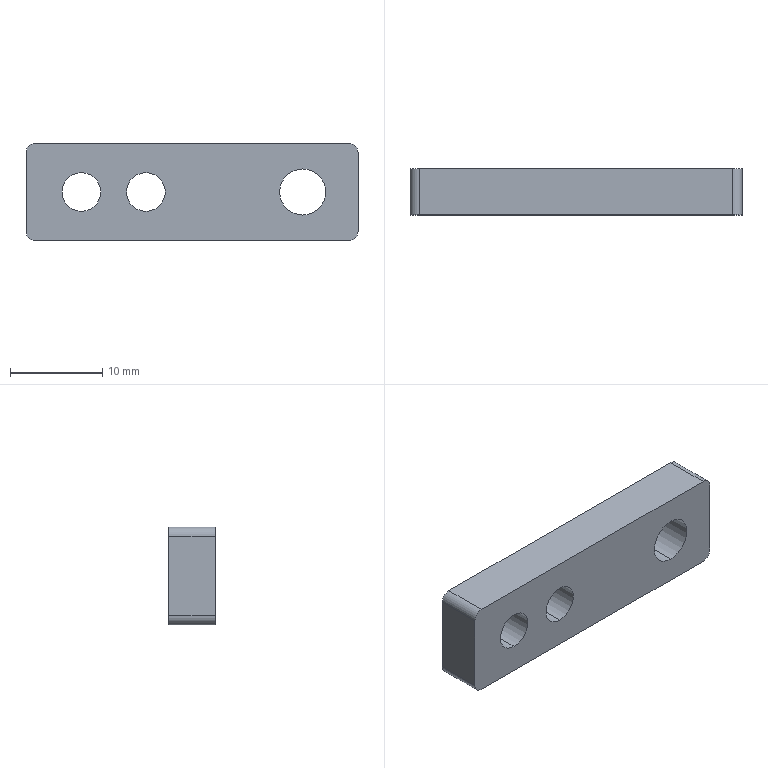Part | STEP file | Driven guide wheel connector | 1 solid | 16 faces | box 36 x 5 x 10.6 mm | volume 1667 mm3 | cylinder 10 | plane 6 | commonest cylinder face diameters 2 x4 4.2 x4 5 x2
STEP:
#1=CARTESIAN_POINT('',(0.,0.,0.));
#2=DIRECTION('',(0.,0.,1.));
#3=DIRECTION('',(1.,0.,0.));
#4=AXIS2_PLACEMENT_3D('',#1,#2,#3);
#5=CARTESIAN_POINT('',(12.,-5.,2.5));
#6=VERTEX_POINT('',#5);
#7=CARTESIAN_POINT('',(12.,0.,2.5));
#8=VERTEX_POINT('',#7);
#9=CARTESIAN_POINT('',(12.,0.,2.5));
#10=DIRECTION('',(0.,1.,0.));
#11=VECTOR('',#10,1.);
#12=LINE('',#9,#11);
#13=CARTESIAN_POINT('',(12.,0.,0.));
#14=DIRECTION('',(0.,1.,0.));
#15=DIRECTION('',(0.,0.,1.));
#16=AXIS2_PLACEMENT_3D('',#13,#14,#15);
#17=CYLINDRICAL_SURFACE('',#16,2.5);
#18=CARTESIAN_POINT('',(6.283,0.));
#19=DIRECTION('',(0.,1.));
#20=VECTOR('',#19,1.);
#21=LINE('',#18,#20);
#22=(GEOMETRIC_REPRESENTATION_CONTEXT(2)PARAMETRIC_REPRESENTATION_CONTEXT()REPRESENTATION_CONTEXT('',''));
#23=DEFINITIONAL_REPRESENTATION('',(#21),#22);
#24=PCURVE('',#17,#23);
#25=CARTESIAN_POINT('',(12.,0.,0.));
#26=DIRECTION('',(0.,1.,0.));
#27=DIRECTION('',(0.,0.,1.));
#28=AXIS2_PLACEMENT_3D('',#25,#26,#27);
#29=CYLINDRICAL_SURFACE('',#28,2.5);
#30=CARTESIAN_POINT('',(0.,0.));
#31=DIRECTION('',(0.,1.));
#32=VECTOR('',#31,1.);
#33=LINE('',#30,#32);
#34=(GEOMETRIC_REPRESENTATION_CONTEXT(2)PARAMETRIC_REPRESENTATION_CONTEXT()REPRESENTATION_CONTEXT('',''));
#35=DEFINITIONAL_REPRESENTATION('',(#33),#34);
#36=PCURVE('',#29,#35);
#37=SURFACE_CURVE('',#12,(#24,#36),.PCURVE_S1.);
#38=EDGE_CURVE('',#6,#8,#37,.T.);
#39=ORIENTED_EDGE('',*,*,#38,.T.);
#40=CARTESIAN_POINT('',(12.,0.,-2.5));
#41=VERTEX_POINT('',#40);
#42=CARTESIAN_POINT('',(12.,0.,0.));
#43=DIRECTION('',(0.,1.,0.));
#44=DIRECTION('',(0.,0.,1.));
#45=AXIS2_PLACEMENT_3D('',#42,#43,#44);
#46=CIRCLE('',#45,2.5);
#47=CARTESIAN_POINT('',(0.,0.));
#48=DIRECTION('',(1.,0.));
#49=VECTOR('',#48,1.);
#50=LINE('',#47,#49);
#51=(GEOMETRIC_REPRESENTATION_CONTEXT(2)PARAMETRIC_REPRESENTATION_CONTEXT()REPRESENTATION_CONTEXT('',''));
#52=DEFINITIONAL_REPRESENTATION('',(#50),#51);
#53=PCURVE('',#17,#52);
#54=CARTESIAN_POINT('',(0.,0.,0.));
#55=DIRECTION('',(0.,1.,0.));
#56=DIRECTION('',(0.,0.,1.));
#57=AXIS2_PLACEMENT_3D('',#54,#55,#56);
#58=PLANE('',#57);
#59=CARTESIAN_POINT('',(0.,12.));
#60=DIRECTION('',(1.,0.));
#61=AXIS2_PLACEMENT_2D('',#59,#60);
#62=CIRCLE('',#61,2.5);
#63=(GEOMETRIC_REPRESENTATION_CONTEXT(2)PARAMETRIC_REPRESENTATION_CONTEXT()REPRESENTATION_CONTEXT('',''));
#64=DEFINITIONAL_REPRESENTATION('',(#62),#63);
#65=PCURVE('',#58,#64);
#66=SURFACE_CURVE('',#46,(#53,#65),.PCURVE_S1.);
#67=EDGE_CURVE('',#41,#8,#66,.T.);
#68=ORIENTED_EDGE('',*,*,#67,.F.);
#69=CARTESIAN_POINT('',(12.,-5.,-2.5));
#70=VERTEX_POINT('',#69);
#71=CARTESIAN_POINT('',(12.,0.,-2.5));
#72=DIRECTION('',(0.,1.,0.));
#73=VECTOR('',#72,1.);
#74=LINE('',#71,#73);
#75=CARTESIAN_POINT('',(3.142,0.));
#76=DIRECTION('',(0.,1.));
#77=VECTOR('',#76,1.);
#78=LINE('',#75,#77);
#79=(GEOMETRIC_REPRESENTATION_CONTEXT(2)PARAMETRIC_REPRESENTATION_CONTEXT()REPRESENTATION_CONTEXT('',''));
#80=DEFINITIONAL_REPRESENTATION('',(#78),#79);
#81=PCURVE('',#17,#80);
#82=CARTESIAN_POINT('',(3.142,0.));
#83=DIRECTION('',(0.,1.));
#84=VECTOR('',#83,1.);
#85=LINE('',#82,#84);
#86=(GEOMETRIC_REPRESENTATION_CONTEXT(2)PARAMETRIC_REPRESENTATION_CONTEXT()REPRESENTATION_CONTEXT('',''));
#87=DEFINITIONAL_REPRESENTATION('',(#85),#86);
#88=PCURVE('',#29,#87);
#89=SURFACE_CURVE('',#74,(#81,#88),.PCURVE_S1.);
#90=EDGE_CURVE('',#70,#41,#89,.T.);
#91=ORIENTED_EDGE('',*,*,#90,.F.);
#92=CARTESIAN_POINT('',(12.,-5.,0.));
#93=DIRECTION('',(0.,1.,0.));
#94=DIRECTION('',(0.,0.,1.));
#95=AXIS2_PLACEMENT_3D('',#92,#93,#94);
#96=CIRCLE('',#95,2.5);
#97=CARTESIAN_POINT('',(0.,-5.));
#98=DIRECTION('',(1.,0.));
#99=VECTOR('',#98,1.);
#100=LINE('',#97,#99);
#101=(GEOMETRIC_REPRESENTATION_CONTEXT(2)PARAMETRIC_REPRESENTATION_CONTEXT()REPRESENTATION_CONTEXT('',''));
#102=DEFINITIONAL_REPRESENTATION('',(#100),#101);
#103=PCURVE('',#17,#102);
#104=CARTESIAN_POINT('',(0.,-5.,0.));
#105=DIRECTION('',(0.,1.,0.));
#106=DIRECTION('',(0.,0.,1.));
#107=AXIS2_PLACEMENT_3D('',#104,#105,#106);
#108=PLANE('',#107);
#109=CARTESIAN_POINT('',(0.,12.));
#110=DIRECTION('',(1.,0.));
#111=AXIS2_PLACEMENT_2D('',#109,#110);
#112=CIRCLE('',#111,2.5);
#113=(GEOMETRIC_REPRESENTATION_CONTEXT(2)PARAMETRIC_REPRESENTATION_CONTEXT()REPRESENTATION_CONTEXT('',''));
#114=DEFINITIONAL_REPRESENTATION('',(#112),#113);
#115=PCURVE('',#108,#114);
#116=SURFACE_CURVE('',#96,(#103,#115),.PCURVE_S1.);
#117=EDGE_CURVE('',#70,#6,#116,.T.);
#118=ORIENTED_EDGE('',*,*,#117,.T.);
#119=EDGE_LOOP('',(#39,#68,#91,#118));
#120=FACE_BOUND('',#119,.F.);
#121=ADVANCED_FACE('',(#120),#17,.F.);
#122=CARTESIAN_POINT('',(-5.,-5.,2.1));
#123=VERTEX_POINT('',#122);
#124=CARTESIAN_POINT('',(-5.,0.,2.1));
#125=VERTEX_POINT('',#124);
#126=CARTESIAN_POINT('',(-5.,0.,2.1));
#127=DIRECTION('',(0.,1.,0.));
#128=VECTOR('',#127,1.);
#129=LINE('',#126,#128);
#130=CARTESIAN_POINT('',(-5.,0.,0.));
#131=DIRECTION('',(0.,1.,0.));
#132=DIRECTION('',(0.,0.,1.));
#133=AXIS2_PLACEMENT_3D('',#130,#131,#132);
#134=CYLINDRICAL_SURFACE('',#133,2.1);
#135=CARTESIAN_POINT('',(6.283,0.));
#136=DIRECTION('',(0.,1.));
#137=VECTOR('',#136,1.);
#138=LINE('',#135,#137);
#139=(GEOMETRIC_REPRESENTATION_CONTEXT(2)PARAMETRIC_REPRESENTATION_CONTEXT()REPRESENTATION_CONTEXT('',''));
#140=DEFINITIONAL_REPRESENTATION('',(#138),#139);
#141=PCURVE('',#134,#140);
#142=CARTESIAN_POINT('',(-5.,0.,0.));
#143=DIRECTION('',(0.,1.,0.));
#144=DIRECTION('',(0.,0.,1.));
#145=AXIS2_PLACEMENT_3D('',#142,#143,#144);
#146=CYLINDRICAL_SURFACE('',#145,2.1);
#147=CARTESIAN_POINT('',(0.,0.));
#148=DIRECTION('',(0.,1.));
#149=VECTOR('',#148,1.);
#150=LINE('',#147,#149);
#151=(GEOMETRIC_REPRESENTATION_CONTEXT(2)PARAMETRIC_REPRESENTATION_CONTEXT()REPRESENTATION_CONTEXT('',''));
#152=DEFINITIONAL_REPRESENTATION('',(#150),#151);
#153=PCURVE('',#146,#152);
#154=SURFACE_CURVE('',#129,(#141,#153),.PCURVE_S1.);
#155=EDGE_CURVE('',#123,#125,#154,.T.);
#156=ORIENTED_EDGE('',*,*,#155,.T.);
#157=CARTESIAN_POINT('',(-5.,0.,-2.1));
#158=VERTEX_POINT('',#157);
#159=CARTESIAN_POINT('',(-5.,0.,0.));
#160=DIRECTION('',(0.,1.,0.));
#161=DIRECTION('',(0.,0.,1.));
#162=AXIS2_PLACEMENT_3D('',#159,#160,#161);
#163=CIRCLE('',#162,2.1);
#164=CARTESIAN_POINT('',(0.,0.));
#165=DIRECTION('',(1.,0.));
#166=VECTOR('',#165,1.);
#167=LINE('',#164,#166);
#168=(GEOMETRIC_REPRESENTATION_CONTEXT(2)PARAMETRIC_REPRESENTATION_CONTEXT()REPRESENTATION_CONTEXT('',''));
#169=DEFINITIONAL_REPRESENTATION('',(#167),#168);
#170=PCURVE('',#134,#169);
#171=CARTESIAN_POINT('',(0.,-5.));
#172=DIRECTION('',(1.,0.));
#173=AXIS2_PLACEMENT_2D('',#171,#172);
#174=CIRCLE('',#173,2.1);
#175=(GEOMETRIC_REPRESENTATION_CONTEXT(2)PARAMETRIC_REPRESENTATION_CONTEXT()REPRESENTATION_CONTEXT('',''));
#176=DEFINITIONAL_REPRESENTATION('',(#174),#175);
#177=PCURVE('',#58,#176);
#178=SURFACE_CURVE('',#163,(#170,#177),.PCURVE_S1.);
#179=EDGE_CURVE('',#158,#125,#178,.T.);
#180=ORIENTED_EDGE('',*,*,#179,.F.);
#181=CARTESIAN_POINT('',(-5.,-5.,-2.1));
#182=VERTEX_POINT('',#181);
#183=CARTESIAN_POINT('',(-5.,0.,-2.1));
#184=DIRECTION('',(0.,1.,0.));
#185=VECTOR('',#184,1.);
#186=LINE('',#183,#185);
#187=CARTESIAN_POINT('',(3.142,0.));
#188=DIRECTION('',(0.,1.));
#189=VECTOR('',#188,1.);
#190=LINE('',#187,#189);
#191=(GEOMETRIC_REPRESENTATION_CONTEXT(2)PARAMETRIC_REPRESENTATION_CONTEXT()REPRESENTATION_CONTEXT('',''));
#192=DEFINITIONAL_REPRESENTATION('',(#190),#191);
#193=PCURVE('',#134,#192);
#194=CARTESIAN_POINT('',(3.142,0.));
#195=DIRECTION('',(0.,1.));
#196=VECTOR('',#195,1.);
#197=LINE('',#194,#196);
#198=(GEOMETRIC_REPRESENTATION_CONTEXT(2)PARAMETRIC_REPRESENTATION_CONTEXT()REPRESENTATION_CONTEXT('',''));
#199=DEFINITIONAL_REPRESENTATION('',(#197),#198);
#200=PCURVE('',#146,#199);
#201=SURFACE_CURVE('',#186,(#193,#200),.PCURVE_S1.);
#202=EDGE_CURVE('',#182,#158,#201,.T.);
#203=ORIENTED_EDGE('',*,*,#202,.F.);
#204=CARTESIAN_POINT('',(-5.,-5.,0.));
#205=DIRECTION('',(0.,1.,0.));
#206=DIRECTION('',(0.,0.,1.));
#207=AXIS2_PLACEMENT_3D('',#204,#205,#206);
#208=CIRCLE('',#207,2.1);
#209=CARTESIAN_POINT('',(0.,-5.));
#210=DIRECTION('',(1.,0.));
#211=VECTOR('',#210,1.);
#212=LINE('',#209,#211);
#213=(GEOMETRIC_REPRESENTATION_CONTEXT(2)PARAMETRIC_REPRESENTATION_CONTEXT()REPRESENTATION_CONTEXT('',''));
#214=DEFINITIONAL_REPRESENTATION('',(#212),#213);
#215=PCURVE('',#134,#214);
#216=CARTESIAN_POINT('',(0.,-5.));
#217=DIRECTION('',(1.,0.));
#218=AXIS2_PLACEMENT_2D('',#216,#217);
#219=CIRCLE('',#218,2.1);
#220=(GEOMETRIC_REPRESENTATION_CONTEXT(2)PARAMETRIC_REPRESENTATION_CONTEXT()REPRESENTATION_CONTEXT('',''));
#221=DEFINITIONAL_REPRESENTATION('',(#219),#220);
#222=PCURVE('',#108,#221);
#223=SURFACE_CURVE('',#208,(#215,#222),.PCURVE_S1.);
#224=EDGE_CURVE('',#182,#123,#223,.T.);
#225=ORIENTED_EDGE('',*,*,#224,.T.);
#226=EDGE_LOOP('',(#156,#180,#203,#225));
#227=FACE_BOUND('',#226,.F.);
#228=ADVANCED_FACE('',(#227),#134,.F.);
#229=CARTESIAN_POINT('',(-12.,-5.,2.1));
#230=VERTEX_POINT('',#229);
#231=CARTESIAN_POINT('',(-12.,0.,2.1));
#232=VERTEX_POINT('',#231);
#233=CARTESIAN_POINT('',(-12.,0.,2.1));
#234=DIRECTION('',(0.,1.,0.));
#235=VECTOR('',#234,1.);
#236=LINE('',#233,#235);
#237=CARTESIAN_POINT('',(-12.,0.,0.));
#238=DIRECTION('',(0.,1.,0.));
#239=DIRECTION('',(0.,0.,1.));
#240=AXIS2_PLACEMENT_3D('',#237,#238,#239);
#241=CYLINDRICAL_SURFACE('',#240,2.1);
#242=CARTESIAN_POINT('',(6.283,0.));
#243=DIRECTION('',(0.,1.));
#244=VECTOR('',#243,1.);
#245=LINE('',#242,#244);
#246=(GEOMETRIC_REPRESENTATION_CONTEXT(2)PARAMETRIC_REPRESENTATION_CONTEXT()REPRESENTATION_CONTEXT('',''));
#247=DEFINITIONAL_REPRESENTATION('',(#245),#246);
#248=PCURVE('',#241,#247);
#249=CARTESIAN_POINT('',(-12.,0.,0.));
#250=DIRECTION('',(0.,1.,0.));
#251=DIRECTION('',(0.,0.,1.));
#252=AXIS2_PLACEMENT_3D('',#249,#250,#251);
#253=CYLINDRICAL_SURFACE('',#252,2.1);
#254=CARTESIAN_POINT('',(0.,0.));
#255=DIRECTION('',(0.,1.));
#256=VECTOR('',#255,1.);
#257=LINE('',#254,#256);
#258=(GEOMETRIC_REPRESENTATION_CONTEXT(2)PARAMETRIC_REPRESENTATION_CONTEXT()REPRESENTATION_CONTEXT('',''));
#259=DEFINITIONAL_REPRESENTATION('',(#257),#258);
#260=PCURVE('',#253,#259);
#261=SURFACE_CURVE('',#236,(#248,#260),.PCURVE_S1.);
#262=EDGE_CURVE('',#230,#232,#261,.T.);
#263=ORIENTED_EDGE('',*,*,#262,.T.);
#264=CARTESIAN_POINT('',(-12.,0.,-2.1));
#265=VERTEX_POINT('',#264);
#266=CARTESIAN_POINT('',(-12.,0.,0.));
#267=DIRECTION('',(0.,1.,0.));
#268=DIRECTION('',(0.,0.,1.));
#269=AXIS2_PLACEMENT_3D('',#266,#267,#268);
#270=CIRCLE('',#269,2.1);
#271=CARTESIAN_POINT('',(0.,0.));
#272=DIRECTION('',(1.,0.));
#273=VECTOR('',#272,1.);
#274=LINE('',#271,#273);
#275=(GEOMETRIC_REPRESENTATION_CONTEXT(2)PARAMETRIC_REPRESENTATION_CONTEXT()REPRESENTATION_CONTEXT('',''));
#276=DEFINITIONAL_REPRESENTATION('',(#274),#275);
#277=PCURVE('',#241,#276);
#278=CARTESIAN_POINT('',(0.,-12.));
#279=DIRECTION('',(1.,0.));
#280=AXIS2_PLACEMENT_2D('',#278,#279);
#281=CIRCLE('',#280,2.1);
#282=(GEOMETRIC_REPRESENTATION_CONTEXT(2)PARAMETRIC_REPRESENTATION_CONTEXT()REPRESENTATION_CONTEXT('',''));
#283=DEFINITIONAL_REPRESENTATION('',(#281),#282);
#284=PCURVE('',#58,#283);
#285=SURFACE_CURVE('',#270,(#277,#284),.PCURVE_S1.);
#286=EDGE_CURVE('',#265,#232,#285,.T.);
#287=ORIENTED_EDGE('',*,*,#286,.F.);
#288=CARTESIAN_POINT('',(-12.,-5.,-2.1));
#289=VERTEX_POINT('',#288);
#290=CARTESIAN_POINT('',(-12.,0.,-2.1));
#291=DIRECTION('',(0.,1.,0.));
#292=VECTOR('',#291,1.);
#293=LINE('',#290,#292);
#294=CARTESIAN_POINT('',(3.142,0.));
#295=DIRECTION('',(0.,1.));
#296=VECTOR('',#295,1.);
#297=LINE('',#294,#296);
#298=(GEOMETRIC_REPRESENTATION_CONTEXT(2)PARAMETRIC_REPRESENTATION_CONTEXT()REPRESENTATION_CONTEXT('',''));
#299=DEFINITIONAL_REPRESENTATION('',(#297),#298);
#300=PCURVE('',#241,#299);
#301=CARTESIAN_POINT('',(3.142,0.));
#302=DIRECTION('',(0.,1.));
#303=VECTOR('',#302,1.);
#304=LINE('',#301,#303);
#305=(GEOMETRIC_REPRESENTATION_CONTEXT(2)PARAMETRIC_REPRESENTATION_CONTEXT()REPRESENTATION_CONTEXT('',''));
#306=DEFINITIONAL_REPRESENTATION('',(#304),#305);
#307=PCURVE('',#253,#306);
#308=SURFACE_CURVE('',#293,(#300,#307),.PCURVE_S1.);
#309=EDGE_CURVE('',#289,#265,#308,.T.);
#310=ORIENTED_EDGE('',*,*,#309,.F.);
#311=CARTESIAN_POINT('',(-12.,-5.,0.));
#312=DIRECTION('',(0.,1.,0.));
#313=DIRECTION('',(0.,0.,1.));
#314=AXIS2_PLACEMENT_3D('',#311,#312,#313);
#315=CIRCLE('',#314,2.1);
#316=CARTESIAN_POINT('',(0.,-5.));
#317=DIRECTION('',(1.,0.));
#318=VECTOR('',#317,1.);
#319=LINE('',#316,#318);
#320=(GEOMETRIC_REPRESENTATION_CONTEXT(2)PARAMETRIC_REPRESENTATION_CONTEXT()REPRESENTATION_CONTEXT('',''));
#321=DEFINITIONAL_REPRESENTATION('',(#319),#320);
#322=PCURVE('',#241,#321);
#323=CARTESIAN_POINT('',(0.,-12.));
#324=DIRECTION('',(1.,0.));
#325=AXIS2_PLACEMENT_2D('',#323,#324);
#326=CIRCLE('',#325,2.1);
#327=(GEOMETRIC_REPRESENTATION_CONTEXT(2)PARAMETRIC_REPRESENTATION_CONTEXT()REPRESENTATION_CONTEXT('',''));
#328=DEFINITIONAL_REPRESENTATION('',(#326),#327);
#329=PCURVE('',#108,#328);
#330=SURFACE_CURVE('',#315,(#322,#329),.PCURVE_S1.);
#331=EDGE_CURVE('',#289,#230,#330,.T.);
#332=ORIENTED_EDGE('',*,*,#331,.T.);
#333=EDGE_LOOP('',(#263,#287,#310,#332));
#334=FACE_BOUND('',#333,.F.);
#335=ADVANCED_FACE('',(#334),#241,.F.);
#336=CARTESIAN_POINT('',(18.,0.,4.3));
#337=VERTEX_POINT('',#336);
#338=CARTESIAN_POINT('',(18.,0.,-4.3));
#339=VERTEX_POINT('',#338);
#340=CARTESIAN_POINT('',(18.,0.,-5.3));
#341=DIRECTION('',(0.,0.,-1.));
#342=VECTOR('',#341,1.);
#343=LINE('',#340,#342);
#344=CARTESIAN_POINT('',(18.,-5.,-5.3));
#345=DIRECTION('',(1.,0.,0.));
#346=DIRECTION('',(0.,0.,-1.));
#347=AXIS2_PLACEMENT_3D('',#344,#345,#346);
#348=PLANE('',#347);
#349=CARTESIAN_POINT('',(0.,5.));
#350=DIRECTION('',(1.,0.));
#351=VECTOR('',#350,1.);
#352=LINE('',#349,#351);
#353=(GEOMETRIC_REPRESENTATION_CONTEXT(2)PARAMETRIC_REPRESENTATION_CONTEXT()REPRESENTATION_CONTEXT('',''));
#354=DEFINITIONAL_REPRESENTATION('',(#352),#353);
#355=PCURVE('',#348,#354);
#356=CARTESIAN_POINT('',(-5.3,18.));
#357=DIRECTION('',(-1.,0.));
#358=VECTOR('',#357,1.);
#359=LINE('',#356,#358);
#360=(GEOMETRIC_REPRESENTATION_CONTEXT(2)PARAMETRIC_REPRESENTATION_CONTEXT()REPRESENTATION_CONTEXT('',''));
#361=DEFINITIONAL_REPRESENTATION('',(#359),#360);
#362=PCURVE('',#58,#361);
#363=SURFACE_CURVE('',#343,(#355,#362),.PCURVE_S1.);
#364=EDGE_CURVE('',#337,#339,#363,.T.);
#365=ORIENTED_EDGE('',*,*,#364,.F.);
#366=CARTESIAN_POINT('',(18.,-5.,4.3));
#367=VERTEX_POINT('',#366);
#368=CARTESIAN_POINT('',(18.,-5.,4.3));
#369=DIRECTION('',(0.,-1.,0.));
#370=VECTOR('',#369,1.);
#371=LINE('',#368,#370);
#372=CARTESIAN_POINT('',(-9.6,0.));
#373=DIRECTION('',(0.,-1.));
#374=VECTOR('',#373,1.);
#375=LINE('',#372,#374);
#376=(GEOMETRIC_REPRESENTATION_CONTEXT(2)PARAMETRIC_REPRESENTATION_CONTEXT()REPRESENTATION_CONTEXT('',''));
#377=DEFINITIONAL_REPRESENTATION('',(#375),#376);
#378=PCURVE('',#348,#377);
#379=CARTESIAN_POINT('',(17.,-5.,4.3));
#380=DIRECTION('',(0.,1.,0.));
#381=DIRECTION('',(0.,0.,1.));
#382=AXIS2_PLACEMENT_3D('',#379,#380,#381);
#383=CYLINDRICAL_SURFACE('',#382,1.);
#384=CARTESIAN_POINT('',(1.571,0.));
#385=DIRECTION('',(0.,-1.));
#386=VECTOR('',#385,1.);
#387=LINE('',#384,#386);
#388=(GEOMETRIC_REPRESENTATION_CONTEXT(2)PARAMETRIC_REPRESENTATION_CONTEXT()REPRESENTATION_CONTEXT('',''));
#389=DEFINITIONAL_REPRESENTATION('',(#387),#388);
#390=PCURVE('',#383,#389);
#391=SURFACE_CURVE('',#371,(#378,#390),.PCURVE_S1.);
#392=EDGE_CURVE('',#337,#367,#391,.T.);
#393=ORIENTED_EDGE('',*,*,#392,.T.);
#394=CARTESIAN_POINT('',(18.,-5.,-4.3));
#395=VERTEX_POINT('',#394);
#396=CARTESIAN_POINT('',(18.,-5.,-5.3));
#397=DIRECTION('',(0.,0.,-1.));
#398=VECTOR('',#397,1.);
#399=LINE('',#396,#398);
#400=CARTESIAN_POINT('',(0.,0.));
#401=DIRECTION('',(1.,0.));
#402=VECTOR('',#401,1.);
#403=LINE('',#400,#402);
#404=(GEOMETRIC_REPRESENTATION_CONTEXT(2)PARAMETRIC_REPRESENTATION_CONTEXT()REPRESENTATION_CONTEXT('',''));
#405=DEFINITIONAL_REPRESENTATION('',(#403),#404);
#406=PCURVE('',#348,#405);
#407=CARTESIAN_POINT('',(-5.3,18.));
#408=DIRECTION('',(-1.,0.));
#409=VECTOR('',#408,1.);
#410=LINE('',#407,#409);
#411=(GEOMETRIC_REPRESENTATION_CONTEXT(2)PARAMETRIC_REPRESENTATION_CONTEXT()REPRESENTATION_CONTEXT('',''));
#412=DEFINITIONAL_REPRESENTATION('',(#410),#411);
#413=PCURVE('',#108,#412);
#414=SURFACE_CURVE('',#399,(#406,#413),.PCURVE_S1.);
#415=EDGE_CURVE('',#367,#395,#414,.T.);
#416=ORIENTED_EDGE('',*,*,#415,.T.);
#417=CARTESIAN_POINT('',(18.,-5.,-4.3));
#418=DIRECTION('',(0.,1.,0.));
#419=VECTOR('',#418,1.);
#420=LINE('',#417,#419);
#421=CARTESIAN_POINT('',(-1.,0.));
#422=DIRECTION('',(0.,1.));
#423=VECTOR('',#422,1.);
#424=LINE('',#421,#423);
#425=(GEOMETRIC_REPRESENTATION_CONTEXT(2)PARAMETRIC_REPRESENTATION_CONTEXT()REPRESENTATION_CONTEXT('',''));
#426=DEFINITIONAL_REPRESENTATION('',(#424),#425);
#427=PCURVE('',#348,#426);
#428=CARTESIAN_POINT('',(17.,-5.,-4.3));
#429=DIRECTION('',(0.,1.,0.));
#430=DIRECTION('',(0.,0.,1.));
#431=AXIS2_PLACEMENT_3D('',#428,#429,#430);
#432=CYLINDRICAL_SURFACE('',#431,1.);
#433=CARTESIAN_POINT('',(1.571,0.));
#434=DIRECTION('',(0.,1.));
#435=VECTOR('',#434,1.);
#436=LINE('',#433,#435);
#437=(GEOMETRIC_REPRESENTATION_CONTEXT(2)PARAMETRIC_REPRESENTATION_CONTEXT()REPRESENTATION_CONTEXT('',''));
#438=DEFINITIONAL_REPRESENTATION('',(#436),#437);
#439=PCURVE('',#432,#438);
#440=SURFACE_CURVE('',#420,(#427,#439),.PCURVE_S1.);
#441=EDGE_CURVE('',#395,#339,#440,.T.);
#442=ORIENTED_EDGE('',*,*,#441,.T.);
#443=EDGE_LOOP('',(#365,#393,#416,#442));
#444=FACE_BOUND('',#443,.T.);
#445=ADVANCED_FACE('',(#444),#348,.T.);
#446=CARTESIAN_POINT('',(-17.,0.,5.3));
#447=VERTEX_POINT('',#446);
#448=CARTESIAN_POINT('',(17.,0.,5.3));
#449=VERTEX_POINT('',#448);
#450=CARTESIAN_POINT('',(-18.,0.,5.3));
#451=DIRECTION('',(1.,0.,0.));
#452=VECTOR('',#451,1.);
#453=LINE('',#450,#452);
#454=CARTESIAN_POINT('',(-18.,-5.,5.3));
#455=DIRECTION('',(0.,0.,1.));
#456=DIRECTION('',(1.,0.,0.));
#457=AXIS2_PLACEMENT_3D('',#454,#455,#456);
#458=PLANE('',#457);
#459=CARTESIAN_POINT('',(0.,5.));
#460=DIRECTION('',(1.,0.));
#461=VECTOR('',#460,1.);
#462=LINE('',#459,#461);
#463=(GEOMETRIC_REPRESENTATION_CONTEXT(2)PARAMETRIC_REPRESENTATION_CONTEXT()REPRESENTATION_CONTEXT('',''));
#464=DEFINITIONAL_REPRESENTATION('',(#462),#463);
#465=PCURVE('',#458,#464);
#466=CARTESIAN_POINT('',(5.3,-18.));
#467=DIRECTION('',(0.,1.));
#468=VECTOR('',#467,1.);
#469=LINE('',#466,#468);
#470=(GEOMETRIC_REPRESENTATION_CONTEXT(2)PARAMETRIC_REPRESENTATION_CONTEXT()REPRESENTATION_CONTEXT('',''));
#471=DEFINITIONAL_REPRESENTATION('',(#469),#470);
#472=PCURVE('',#58,#471);
#473=SURFACE_CURVE('',#453,(#465,#472),.PCURVE_S1.);
#474=EDGE_CURVE('',#447,#449,#473,.T.);
#475=ORIENTED_EDGE('',*,*,#474,.F.);
#476=CARTESIAN_POINT('',(-17.,-5.,5.3));
#477=VERTEX_POINT('',#476);
#478=CARTESIAN_POINT('',(-17.,-5.,5.3));
#479=DIRECTION('',(0.,-1.,0.));
#480=VECTOR('',#479,1.);
#481=LINE('',#478,#480);
#482=CARTESIAN_POINT('',(1.,0.));
#483=DIRECTION('',(0.,-1.));
#484=VECTOR('',#483,1.);
#485=LINE('',#482,#484);
#486=(GEOMETRIC_REPRESENTATION_CONTEXT(2)PARAMETRIC_REPRESENTATION_CONTEXT()REPRESENTATION_CONTEXT('',''));
#487=DEFINITIONAL_REPRESENTATION('',(#485),#486);
#488=PCURVE('',#458,#487);
#489=CARTESIAN_POINT('',(-17.,-5.,4.3));
#490=DIRECTION('',(0.,1.,0.));
#491=DIRECTION('',(0.,0.,1.));
#492=AXIS2_PLACEMENT_3D('',#489,#490,#491);
#493=CYLINDRICAL_SURFACE('',#492,1.);
#494=CARTESIAN_POINT('',(6.283,0.));
#495=DIRECTION('',(0.,-1.));
#496=VECTOR('',#495,1.);
#497=LINE('',#494,#496);
#498=(GEOMETRIC_REPRESENTATION_CONTEXT(2)PARAMETRIC_REPRESENTATION_CONTEXT()REPRESENTATION_CONTEXT('',''));
#499=DEFINITIONAL_REPRESENTATION('',(#497),#498);
#500=PCURVE('',#493,#499);
#501=SURFACE_CURVE('',#481,(#488,#500),.PCURVE_S1.);
#502=EDGE_CURVE('',#447,#477,#501,.T.);
#503=ORIENTED_EDGE('',*,*,#502,.T.);
#504=CARTESIAN_POINT('',(17.,-5.,5.3));
#505=VERTEX_POINT('',#504);
#506=CARTESIAN_POINT('',(-18.,-5.,5.3));
#507=DIRECTION('',(1.,0.,0.));
#508=VECTOR('',#507,1.);
#509=LINE('',#506,#508);
#510=CARTESIAN_POINT('',(0.,0.));
#511=DIRECTION('',(1.,0.));
#512=VECTOR('',#511,1.);
#513=LINE('',#510,#512);
#514=(GEOMETRIC_REPRESENTATION_CONTEXT(2)PARAMETRIC_REPRESENTATION_CONTEXT()REPRESENTATION_CONTEXT('',''));
#515=DEFINITIONAL_REPRESENTATION('',(#513),#514);
#516=PCURVE('',#458,#515);
#517=CARTESIAN_POINT('',(5.3,-18.));
#518=DIRECTION('',(0.,1.));
#519=VECTOR('',#518,1.);
#520=LINE('',#517,#519);
#521=(GEOMETRIC_REPRESENTATION_CONTEXT(2)PARAMETRIC_REPRESENTATION_CONTEXT()REPRESENTATION_CONTEXT('',''));
#522=DEFINITIONAL_REPRESENTATION('',(#520),#521);
#523=PCURVE('',#108,#522);
#524=SURFACE_CURVE('',#509,(#516,#523),.PCURVE_S1.);
#525=EDGE_CURVE('',#477,#505,#524,.T.);
#526=ORIENTED_EDGE('',*,*,#525,.T.);
#527=CARTESIAN_POINT('',(17.,-5.,5.3));
#528=DIRECTION('',(0.,1.,0.));
#529=VECTOR('',#528,1.);
#530=LINE('',#527,#529);
#531=CARTESIAN_POINT('',(35.,0.));
#532=DIRECTION('',(0.,1.));
#533=VECTOR('',#532,1.);
#534=LINE('',#531,#533);
#535=(GEOMETRIC_REPRESENTATION_CONTEXT(2)PARAMETRIC_REPRESENTATION_CONTEXT()REPRESENTATION_CONTEXT('',''));
#536=DEFINITIONAL_REPRESENTATION('',(#534),#535);
#537=PCURVE('',#458,#536);
#538=CARTESIAN_POINT('',(0.,0.));
#539=DIRECTION('',(0.,1.));
#540=VECTOR('',#539,1.);
#541=LINE('',#538,#540);
#542=(GEOMETRIC_REPRESENTATION_CONTEXT(2)PARAMETRIC_REPRESENTATION_CONTEXT()REPRESENTATION_CONTEXT('',''));
#543=DEFINITIONAL_REPRESENTATION('',(#541),#542);
#544=PCURVE('',#383,#543);
#545=SURFACE_CURVE('',#530,(#537,#544),.PCURVE_S1.);
#546=EDGE_CURVE('',#505,#449,#545,.T.);
#547=ORIENTED_EDGE('',*,*,#546,.T.);
#548=EDGE_LOOP('',(#475,#503,#526,#547));
#549=FACE_BOUND('',#548,.T.);
#550=ADVANCED_FACE('',(#549),#458,.T.);
#551=CARTESIAN_POINT('',(-18.,-5.,-4.3));
#552=VERTEX_POINT('',#551);
#553=CARTESIAN_POINT('',(-18.,-5.,4.3));
#554=VERTEX_POINT('',#553);
#555=CARTESIAN_POINT('',(-18.,-5.,-5.3));
#556=DIRECTION('',(0.,0.,1.));
#557=VECTOR('',#556,1.);
#558=LINE('',#555,#557);
#559=CARTESIAN_POINT('',(-18.,-5.,-5.3));
#560=DIRECTION('',(-1.,0.,0.));
#561=DIRECTION('',(0.,0.,1.));
#562=AXIS2_PLACEMENT_3D('',#559,#560,#561);
#563=PLANE('',#562);
#564=CARTESIAN_POINT('',(0.,0.));
#565=DIRECTION('',(1.,0.));
#566=VECTOR('',#565,1.);
#567=LINE('',#564,#566);
#568=(GEOMETRIC_REPRESENTATION_CONTEXT(2)PARAMETRIC_REPRESENTATION_CONTEXT()REPRESENTATION_CONTEXT('',''));
#569=DEFINITIONAL_REPRESENTATION('',(#567),#568);
#570=PCURVE('',#563,#569);
#571=CARTESIAN_POINT('',(-5.3,-18.));
#572=DIRECTION('',(1.,0.));
#573=VECTOR('',#572,1.);
#574=LINE('',#571,#573);
#575=(GEOMETRIC_REPRESENTATION_CONTEXT(2)PARAMETRIC_REPRESENTATION_CONTEXT()REPRESENTATION_CONTEXT('',''));
#576=DEFINITIONAL_REPRESENTATION('',(#574),#575);
#577=PCURVE('',#108,#576);
#578=SURFACE_CURVE('',#558,(#570,#577),.PCURVE_S1.);
#579=EDGE_CURVE('',#552,#554,#578,.T.);
#580=ORIENTED_EDGE('',*,*,#579,.T.);
#581=CARTESIAN_POINT('',(-18.,0.,4.3));
#582=VERTEX_POINT('',#581);
#583=CARTESIAN_POINT('',(-18.,-5.,4.3));
#584=DIRECTION('',(0.,1.,0.));
#585=VECTOR('',#584,1.);
#586=LINE('',#583,#585);
#587=CARTESIAN_POINT('',(9.6,0.));
#588=DIRECTION('',(0.,1.));
#589=VECTOR('',#588,1.);
#590=LINE('',#587,#589);
#591=(GEOMETRIC_REPRESENTATION_CONTEXT(2)PARAMETRIC_REPRESENTATION_CONTEXT()REPRESENTATION_CONTEXT('',''));
#592=DEFINITIONAL_REPRESENTATION('',(#590),#591);
#593=PCURVE('',#563,#592);
#594=CARTESIAN_POINT('',(4.712,0.));
#595=DIRECTION('',(0.,1.));
#596=VECTOR('',#595,1.);
#597=LINE('',#594,#596);
#598=(GEOMETRIC_REPRESENTATION_CONTEXT(2)PARAMETRIC_REPRESENTATION_CONTEXT()REPRESENTATION_CONTEXT('',''));
#599=DEFINITIONAL_REPRESENTATION('',(#597),#598);
#600=PCURVE('',#493,#599);
#601=SURFACE_CURVE('',#586,(#593,#600),.PCURVE_S1.);
#602=EDGE_CURVE('',#554,#582,#601,.T.);
#603=ORIENTED_EDGE('',*,*,#602,.T.);
#604=CARTESIAN_POINT('',(-18.,0.,-4.3));
#605=VERTEX_POINT('',#604);
#606=CARTESIAN_POINT('',(-18.,0.,-5.3));
#607=DIRECTION('',(0.,0.,1.));
#608=VECTOR('',#607,1.);
#609=LINE('',#606,#608);
#610=CARTESIAN_POINT('',(0.,5.));
#611=DIRECTION('',(1.,0.));
#612=VECTOR('',#611,1.);
#613=LINE('',#610,#612);
#614=(GEOMETRIC_REPRESENTATION_CONTEXT(2)PARAMETRIC_REPRESENTATION_CONTEXT()REPRESENTATION_CONTEXT('',''));
#615=DEFINITIONAL_REPRESENTATION('',(#613),#614);
#616=PCURVE('',#563,#615);
#617=CARTESIAN_POINT('',(-5.3,-18.));
#618=DIRECTION('',(1.,0.));
#619=VECTOR('',#618,1.);
#620=LINE('',#617,#619);
#621=(GEOMETRIC_REPRESENTATION_CONTEXT(2)PARAMETRIC_REPRESENTATION_CONTEXT()REPRESENTATION_CONTEXT('',''));
#622=DEFINITIONAL_REPRESENTATION('',(#620),#621);
#623=PCURVE('',#58,#622);
#624=SURFACE_CURVE('',#609,(#616,#623),.PCURVE_S1.);
#625=EDGE_CURVE('',#605,#582,#624,.T.);
#626=ORIENTED_EDGE('',*,*,#625,.F.);
#627=CARTESIAN_POINT('',(-18.,-5.,-4.3));
#628=DIRECTION('',(0.,-1.,0.));
#629=VECTOR('',#628,1.);
#630=LINE('',#627,#629);
#631=CARTESIAN_POINT('',(1.,0.));
#632=DIRECTION('',(0.,-1.));
#633=VECTOR('',#632,1.);
#634=LINE('',#631,#633);
#635=(GEOMETRIC_REPRESENTATION_CONTEXT(2)PARAMETRIC_REPRESENTATION_CONTEXT()REPRESENTATION_CONTEXT('',''));
#636=DEFINITIONAL_REPRESENTATION('',(#634),#635);
#637=PCURVE('',#563,#636);
#638=CARTESIAN_POINT('',(-17.,-5.,-4.3));
#639=DIRECTION('',(0.,1.,0.));
#640=DIRECTION('',(0.,0.,1.));
#641=AXIS2_PLACEMENT_3D('',#638,#639,#640);
#642=CYLINDRICAL_SURFACE('',#641,1.);
#643=CARTESIAN_POINT('',(4.712,0.));
#644=DIRECTION('',(0.,-1.));
#645=VECTOR('',#644,1.);
#646=LINE('',#643,#645);
#647=(GEOMETRIC_REPRESENTATION_CONTEXT(2)PARAMETRIC_REPRESENTATION_CONTEXT()REPRESENTATION_CONTEXT('',''));
#648=DEFINITIONAL_REPRESENTATION('',(#646),#647);
#649=PCURVE('',#642,#648);
#650=SURFACE_CURVE('',#630,(#637,#649),.PCURVE_S1.);
#651=EDGE_CURVE('',#605,#552,#650,.T.);
#652=ORIENTED_EDGE('',*,*,#651,.T.);
#653=EDGE_LOOP('',(#580,#603,#626,#652));
#654=FACE_BOUND('',#653,.T.);
#655=ADVANCED_FACE('',(#654),#563,.T.);
#656=CARTESIAN_POINT('',(17.,0.,-5.3));
#657=VERTEX_POINT('',#656);
#658=CARTESIAN_POINT('',(-17.,0.,-5.3));
#659=VERTEX_POINT('',#658);
#660=CARTESIAN_POINT('',(-18.,0.,-5.3));
#661=DIRECTION('',(-1.,0.,0.));
#662=VECTOR('',#661,1.);
#663=LINE('',#660,#662);
#664=CARTESIAN_POINT('',(-18.,-5.,-5.3));
#665=DIRECTION('',(0.,0.,-1.));
#666=DIRECTION('',(-1.,0.,0.));
#667=AXIS2_PLACEMENT_3D('',#664,#665,#666);
#668=PLANE('',#667);
#669=CARTESIAN_POINT('',(0.,5.));
#670=DIRECTION('',(1.,0.));
#671=VECTOR('',#670,1.);
#672=LINE('',#669,#671);
#673=(GEOMETRIC_REPRESENTATION_CONTEXT(2)PARAMETRIC_REPRESENTATION_CONTEXT()REPRESENTATION_CONTEXT('',''));
#674=DEFINITIONAL_REPRESENTATION('',(#672),#673);
#675=PCURVE('',#668,#674);
#676=CARTESIAN_POINT('',(-5.3,-18.));
#677=DIRECTION('',(0.,-1.));
#678=VECTOR('',#677,1.);
#679=LINE('',#676,#678);
#680=(GEOMETRIC_REPRESENTATION_CONTEXT(2)PARAMETRIC_REPRESENTATION_CONTEXT()REPRESENTATION_CONTEXT('',''));
#681=DEFINITIONAL_REPRESENTATION('',(#679),#680);
#682=PCURVE('',#58,#681);
#683=SURFACE_CURVE('',#663,(#675,#682),.PCURVE_S1.);
#684=EDGE_CURVE('',#657,#659,#683,.T.);
#685=ORIENTED_EDGE('',*,*,#684,.F.);
#686=CARTESIAN_POINT('',(17.,-5.,-5.3));
#687=VERTEX_POINT('',#686);
#688=CARTESIAN_POINT('',(17.,-5.,-5.3));
#689=DIRECTION('',(0.,-1.,0.));
#690=VECTOR('',#689,1.);
#691=LINE('',#688,#690);
#692=CARTESIAN_POINT('',(-35.,0.));
#693=DIRECTION('',(0.,-1.));
#694=VECTOR('',#693,1.);
#695=LINE('',#692,#694);
#696=(GEOMETRIC_REPRESENTATION_CONTEXT(2)PARAMETRIC_REPRESENTATION_CONTEXT()REPRESENTATION_CONTEXT('',''));
#697=DEFINITIONAL_REPRESENTATION('',(#695),#696);
#698=PCURVE('',#668,#697);
#699=CARTESIAN_POINT('',(3.142,0.));
#700=DIRECTION('',(0.,-1.));
#701=VECTOR('',#700,1.);
#702=LINE('',#699,#701);
#703=(GEOMETRIC_REPRESENTATION_CONTEXT(2)PARAMETRIC_REPRESENTATION_CONTEXT()REPRESENTATION_CONTEXT('',''));
#704=DEFINITIONAL_REPRESENTATION('',(#702),#703);
#705=PCURVE('',#432,#704);
#706=SURFACE_CURVE('',#691,(#698,#705),.PCURVE_S1.);
#707=EDGE_CURVE('',#657,#687,#706,.T.);
#708=ORIENTED_EDGE('',*,*,#707,.T.);
#709=CARTESIAN_POINT('',(-17.,-5.,-5.3));
#710=VERTEX_POINT('',#709);
#711=CARTESIAN_POINT('',(-18.,-5.,-5.3));
#712=DIRECTION('',(-1.,0.,0.));
#713=VECTOR('',#712,1.);
#714=LINE('',#711,#713);
#715=CARTESIAN_POINT('',(0.,0.));
#716=DIRECTION('',(1.,0.));
#717=VECTOR('',#716,1.);
#718=LINE('',#715,#717);
#719=(GEOMETRIC_REPRESENTATION_CONTEXT(2)PARAMETRIC_REPRESENTATION_CONTEXT()REPRESENTATION_CONTEXT('',''));
#720=DEFINITIONAL_REPRESENTATION('',(#718),#719);
#721=PCURVE('',#668,#720);
#722=CARTESIAN_POINT('',(-5.3,-18.));
#723=DIRECTION('',(0.,-1.));
#724=VECTOR('',#723,1.);
#725=LINE('',#722,#724);
#726=(GEOMETRIC_REPRESENTATION_CONTEXT(2)PARAMETRIC_REPRESENTATION_CONTEXT()REPRESENTATION_CONTEXT('',''));
#727=DEFINITIONAL_REPRESENTATION('',(#725),#726);
#728=PCURVE('',#108,#727);
#729=SURFACE_CURVE('',#714,(#721,#728),.PCURVE_S1.);
#730=EDGE_CURVE('',#687,#710,#729,.T.);
#731=ORIENTED_EDGE('',*,*,#730,.T.);
#732=CARTESIAN_POINT('',(-17.,-5.,-5.3));
#733=DIRECTION('',(0.,1.,0.));
#734=VECTOR('',#733,1.);
#735=LINE('',#732,#734);
#736=CARTESIAN_POINT('',(-1.,0.));
#737=DIRECTION('',(0.,1.));
#738=VECTOR('',#737,1.);
#739=LINE('',#736,#738);
#740=(GEOMETRIC_REPRESENTATION_CONTEXT(2)PARAMETRIC_REPRESENTATION_CONTEXT()REPRESENTATION_CONTEXT('',''));
#741=DEFINITIONAL_REPRESENTATION('',(#739),#740);
#742=PCURVE('',#668,#741);
#743=CARTESIAN_POINT('',(3.142,0.));
#744=DIRECTION('',(0.,1.));
#745=VECTOR('',#744,1.);
#746=LINE('',#743,#745);
#747=(GEOMETRIC_REPRESENTATION_CONTEXT(2)PARAMETRIC_REPRESENTATION_CONTEXT()REPRESENTATION_CONTEXT('',''));
#748=DEFINITIONAL_REPRESENTATION('',(#746),#747);
#749=PCURVE('',#642,#748);
#750=SURFACE_CURVE('',#735,(#742,#749),.PCURVE_S1.);
#751=EDGE_CURVE('',#710,#659,#750,.T.);
#752=ORIENTED_EDGE('',*,*,#751,.T.);
#753=EDGE_LOOP('',(#685,#708,#731,#752));
#754=FACE_BOUND('',#753,.T.);
#755=ADVANCED_FACE('',(#754),#668,.T.);
#756=CARTESIAN_POINT('',(12.,-5.,0.));
#757=DIRECTION('',(0.,1.,0.));
#758=DIRECTION('',(0.,0.,1.));
#759=AXIS2_PLACEMENT_3D('',#756,#757,#758);
#760=CIRCLE('',#759,2.5);
#761=CARTESIAN_POINT('',(0.,12.));
#762=DIRECTION('',(1.,0.));
#763=AXIS2_PLACEMENT_2D('',#761,#762);
#764=CIRCLE('',#763,2.5);
#765=(GEOMETRIC_REPRESENTATION_CONTEXT(2)PARAMETRIC_REPRESENTATION_CONTEXT()REPRESENTATION_CONTEXT('',''));
#766=DEFINITIONAL_REPRESENTATION('',(#764),#765);
#767=PCURVE('',#108,#766);
#768=CARTESIAN_POINT('',(0.,-5.));
#769=DIRECTION('',(1.,0.));
#770=VECTOR('',#769,1.);
#771=LINE('',#768,#770);
#772=(GEOMETRIC_REPRESENTATION_CONTEXT(2)PARAMETRIC_REPRESENTATION_CONTEXT()REPRESENTATION_CONTEXT('',''));
#773=DEFINITIONAL_REPRESENTATION('',(#771),#772);
#774=PCURVE('',#29,#773);
#775=SURFACE_CURVE('',#760,(#767,#774),.PCURVE_S1.);
#776=EDGE_CURVE('',#6,#70,#775,.T.);
#777=ORIENTED_EDGE('',*,*,#776,.T.);
#778=ORIENTED_EDGE('',*,*,#117,.T.);
#779=EDGE_LOOP('',(#777,#778));
#780=FACE_BOUND('',#779,.T.);
#781=CARTESIAN_POINT('',(-5.,-5.,0.));
#782=DIRECTION('',(0.,1.,0.));
#783=DIRECTION('',(0.,0.,1.));
#784=AXIS2_PLACEMENT_3D('',#781,#782,#783);
#785=CIRCLE('',#784,2.1);
#786=CARTESIAN_POINT('',(0.,-5.));
#787=DIRECTION('',(1.,0.));
#788=AXIS2_PLACEMENT_2D('',#786,#787);
#789=CIRCLE('',#788,2.1);
#790=(GEOMETRIC_REPRESENTATION_CONTEXT(2)PARAMETRIC_REPRESENTATION_CONTEXT()REPRESENTATION_CONTEXT('',''));
#791=DEFINITIONAL_REPRESENTATION('',(#789),#790);
#792=PCURVE('',#108,#791);
#793=CARTESIAN_POINT('',(0.,-5.));
#794=DIRECTION('',(1.,0.));
#795=VECTOR('',#794,1.);
#796=LINE('',#793,#795);
#797=(GEOMETRIC_REPRESENTATION_CONTEXT(2)PARAMETRIC_REPRESENTATION_CONTEXT()REPRESENTATION_CONTEXT('',''));
#798=DEFINITIONAL_REPRESENTATION('',(#796),#797);
#799=PCURVE('',#146,#798);
#800=SURFACE_CURVE('',#785,(#792,#799),.PCURVE_S1.);
#801=EDGE_CURVE('',#123,#182,#800,.T.);
#802=ORIENTED_EDGE('',*,*,#801,.T.);
#803=ORIENTED_EDGE('',*,*,#224,.T.);
#804=EDGE_LOOP('',(#802,#803));
#805=FACE_BOUND('',#804,.T.);
#806=CARTESIAN_POINT('',(-12.,-5.,0.));
#807=DIRECTION('',(0.,1.,0.));
#808=DIRECTION('',(0.,0.,1.));
#809=AXIS2_PLACEMENT_3D('',#806,#807,#808);
#810=CIRCLE('',#809,2.1);
#811=CARTESIAN_POINT('',(0.,-12.));
#812=DIRECTION('',(1.,0.));
#813=AXIS2_PLACEMENT_2D('',#811,#812);
#814=CIRCLE('',#813,2.1);
#815=(GEOMETRIC_REPRESENTATION_CONTEXT(2)PARAMETRIC_REPRESENTATION_CONTEXT()REPRESENTATION_CONTEXT('',''));
#816=DEFINITIONAL_REPRESENTATION('',(#814),#815);
#817=PCURVE('',#108,#816);
#818=CARTESIAN_POINT('',(0.,-5.));
#819=DIRECTION('',(1.,0.));
#820=VECTOR('',#819,1.);
#821=LINE('',#818,#820);
#822=(GEOMETRIC_REPRESENTATION_CONTEXT(2)PARAMETRIC_REPRESENTATION_CONTEXT()REPRESENTATION_CONTEXT('',''));
#823=DEFINITIONAL_REPRESENTATION('',(#821),#822);
#824=PCURVE('',#253,#823);
#825=SURFACE_CURVE('',#810,(#817,#824),.PCURVE_S1.);
#826=EDGE_CURVE('',#230,#289,#825,.T.);
#827=ORIENTED_EDGE('',*,*,#826,.T.);
#828=ORIENTED_EDGE('',*,*,#331,.T.);
#829=EDGE_LOOP('',(#827,#828));
#830=FACE_BOUND('',#829,.T.);
#831=ORIENTED_EDGE('',*,*,#525,.F.);
#832=CARTESIAN_POINT('',(-17.,-5.,4.3));
#833=DIRECTION('',(0.,-1.,0.));
#834=DIRECTION('',(0.,0.,1.));
#835=AXIS2_PLACEMENT_3D('',#832,#833,#834);
#836=CIRCLE('',#835,1.);
#837=CARTESIAN_POINT('',(5.3,-17.));
#838=CARTESIAN_POINT('',(5.3,-18.732));
#839=CARTESIAN_POINT('',(3.8,-17.866));
#840=CARTESIAN_POINT('',(2.3,-17.));
#841=CARTESIAN_POINT('',(3.8,-16.134));
#842=CARTESIAN_POINT('',(5.3,-15.268));
#843=CARTESIAN_POINT('',(5.3,-17.));
#844=(BOUNDED_CURVE()B_SPLINE_CURVE(2,(#837,#838,#839,#840,#841,#842,#843),.UNSPECIFIED.,.T.,.F.)B_SPLINE_CURVE_WITH_KNOTS((1,2,2,2,2,1),(-2.094,0.,2.094,4.189,6.283,8.378),.UNSPECIFIED.)CURVE()GEOMETRIC_REPRESENTATION_ITEM()RATIONAL_B_SPLINE_CURVE((1.,0.5,1.,0.5,1.,0.5,1.))REPRESENTATION_ITEM(''));
#845=(GEOMETRIC_REPRESENTATION_CONTEXT(2)PARAMETRIC_REPRESENTATION_CONTEXT()REPRESENTATION_CONTEXT('',''));
#846=DEFINITIONAL_REPRESENTATION('',(#844),#845);
#847=PCURVE('',#108,#846);
#848=CARTESIAN_POINT('',(6.283,0.));
#849=DIRECTION('',(-1.,0.));
#850=VECTOR('',#849,1.);
#851=LINE('',#848,#850);
#852=(GEOMETRIC_REPRESENTATION_CONTEXT(2)PARAMETRIC_REPRESENTATION_CONTEXT()REPRESENTATION_CONTEXT('',''));
#853=DEFINITIONAL_REPRESENTATION('',(#851),#852);
#854=PCURVE('',#493,#853);
#855=SURFACE_CURVE('',#836,(#847,#854),.PCURVE_S1.);
#856=EDGE_CURVE('',#477,#554,#855,.T.);
#857=ORIENTED_EDGE('',*,*,#856,.T.);
#858=ORIENTED_EDGE('',*,*,#579,.F.);
#859=CARTESIAN_POINT('',(-17.,-5.,-4.3));
#860=DIRECTION('',(0.,-1.,0.));
#861=DIRECTION('',(0.,0.,1.));
#862=AXIS2_PLACEMENT_3D('',#859,#860,#861);
#863=CIRCLE('',#862,1.);
#864=CARTESIAN_POINT('',(-3.3,-17.));
#865=CARTESIAN_POINT('',(-3.3,-18.732));
#866=CARTESIAN_POINT('',(-4.8,-17.866));
#867=CARTESIAN_POINT('',(-6.3,-17.));
#868=CARTESIAN_POINT('',(-4.8,-16.134));
#869=CARTESIAN_POINT('',(-3.3,-15.268));
#870=CARTESIAN_POINT('',(-3.3,-17.));
#871=(BOUNDED_CURVE()B_SPLINE_CURVE(2,(#864,#865,#866,#867,#868,#869,#870),.UNSPECIFIED.,.T.,.F.)B_SPLINE_CURVE_WITH_KNOTS((1,2,2,2,2,1),(-2.094,0.,2.094,4.189,6.283,8.378),.UNSPECIFIED.)CURVE()GEOMETRIC_REPRESENTATION_ITEM()RATIONAL_B_SPLINE_CURVE((1.,0.5,1.,0.5,1.,0.5,1.))REPRESENTATION_ITEM(''));
#872=(GEOMETRIC_REPRESENTATION_CONTEXT(2)PARAMETRIC_REPRESENTATION_CONTEXT()REPRESENTATION_CONTEXT('',''));
#873=DEFINITIONAL_REPRESENTATION('',(#871),#872);
#874=PCURVE('',#108,#873);
#875=CARTESIAN_POINT('',(6.283,0.));
#876=DIRECTION('',(-1.,0.));
#877=VECTOR('',#876,1.);
#878=LINE('',#875,#877);
#879=(GEOMETRIC_REPRESENTATION_CONTEXT(2)PARAMETRIC_REPRESENTATION_CONTEXT()REPRESENTATION_CONTEXT('',''));
#880=DEFINITIONAL_REPRESENTATION('',(#878),#879);
#881=PCURVE('',#642,#880);
#882=SURFACE_CURVE('',#863,(#874,#881),.PCURVE_S1.);
#883=EDGE_CURVE('',#552,#710,#882,.T.);
#884=ORIENTED_EDGE('',*,*,#883,.T.);
#885=ORIENTED_EDGE('',*,*,#730,.F.);
#886=CARTESIAN_POINT('',(17.,-5.,-4.3));
#887=DIRECTION('',(0.,-1.,0.));
#888=DIRECTION('',(0.,0.,1.));
#889=AXIS2_PLACEMENT_3D('',#886,#887,#888);
#890=CIRCLE('',#889,1.);
#891=CARTESIAN_POINT('',(-3.3,17.));
#892=CARTESIAN_POINT('',(-3.3,15.268));
#893=CARTESIAN_POINT('',(-4.8,16.134));
#894=CARTESIAN_POINT('',(-6.3,17.));
#895=CARTESIAN_POINT('',(-4.8,17.866));
#896=CARTESIAN_POINT('',(-3.3,18.732));
#897=CARTESIAN_POINT('',(-3.3,17.));
#898=(BOUNDED_CURVE()B_SPLINE_CURVE(2,(#891,#892,#893,#894,#895,#896,#897),.UNSPECIFIED.,.T.,.F.)B_SPLINE_CURVE_WITH_KNOTS((1,2,2,2,2,1),(-2.094,0.,2.094,4.189,6.283,8.378),.UNSPECIFIED.)CURVE()GEOMETRIC_REPRESENTATION_ITEM()RATIONAL_B_SPLINE_CURVE((1.,0.5,1.,0.5,1.,0.5,1.))REPRESENTATION_ITEM(''));
#899=(GEOMETRIC_REPRESENTATION_CONTEXT(2)PARAMETRIC_REPRESENTATION_CONTEXT()REPRESENTATION_CONTEXT('',''));
#900=DEFINITIONAL_REPRESENTATION('',(#898),#899);
#901=PCURVE('',#108,#900);
#902=CARTESIAN_POINT('',(6.283,0.));
#903=DIRECTION('',(-1.,0.));
#904=VECTOR('',#903,1.);
#905=LINE('',#902,#904);
#906=(GEOMETRIC_REPRESENTATION_CONTEXT(2)PARAMETRIC_REPRESENTATION_CONTEXT()REPRESENTATION_CONTEXT('',''));
#907=DEFINITIONAL_REPRESENTATION('',(#905),#906);
#908=PCURVE('',#432,#907);
#909=SURFACE_CURVE('',#890,(#901,#908),.PCURVE_S1.);
#910=EDGE_CURVE('',#687,#395,#909,.T.);
#911=ORIENTED_EDGE('',*,*,#910,.T.);
#912=ORIENTED_EDGE('',*,*,#415,.F.);
#913=CARTESIAN_POINT('',(17.,-5.,4.3));
#914=DIRECTION('',(0.,-1.,0.));
#915=DIRECTION('',(0.,0.,1.));
#916=AXIS2_PLACEMENT_3D('',#913,#914,#915);
#917=CIRCLE('',#916,1.);
#918=CARTESIAN_POINT('',(5.3,17.));
#919=CARTESIAN_POINT('',(5.3,15.268));
#920=CARTESIAN_POINT('',(3.8,16.134));
#921=CARTESIAN_POINT('',(2.3,17.));
#922=CARTESIAN_POINT('',(3.8,17.866));
#923=CARTESIAN_POINT('',(5.3,18.732));
#924=CARTESIAN_POINT('',(5.3,17.));
#925=(BOUNDED_CURVE()B_SPLINE_CURVE(2,(#918,#919,#920,#921,#922,#923,#924),.UNSPECIFIED.,.T.,.F.)B_SPLINE_CURVE_WITH_KNOTS((1,2,2,2,2,1),(-2.094,0.,2.094,4.189,6.283,8.378),.UNSPECIFIED.)CURVE()GEOMETRIC_REPRESENTATION_ITEM()RATIONAL_B_SPLINE_CURVE((1.,0.5,1.,0.5,1.,0.5,1.))REPRESENTATION_ITEM(''));
#926=(GEOMETRIC_REPRESENTATION_CONTEXT(2)PARAMETRIC_REPRESENTATION_CONTEXT()REPRESENTATION_CONTEXT('',''));
#927=DEFINITIONAL_REPRESENTATION('',(#925),#926);
#928=PCURVE('',#108,#927);
#929=CARTESIAN_POINT('',(6.283,0.));
#930=DIRECTION('',(-1.,0.));
#931=VECTOR('',#930,1.);
#932=LINE('',#929,#931);
#933=(GEOMETRIC_REPRESENTATION_CONTEXT(2)PARAMETRIC_REPRESENTATION_CONTEXT()REPRESENTATION_CONTEXT('',''));
#934=DEFINITIONAL_REPRESENTATION('',(#932),#933);
#935=PCURVE('',#383,#934);
#936=SURFACE_CURVE('',#917,(#928,#935),.PCURVE_S1.);
#937=EDGE_CURVE('',#367,#505,#936,.T.);
#938=ORIENTED_EDGE('',*,*,#937,.T.);
#939=EDGE_LOOP('',(#831,#857,#858,#884,#885,#911,#912,#938));
#940=FACE_BOUND('',#939,.T.);
#941=ADVANCED_FACE('',(#780,#805,#830,#940),#108,.F.);
#942=CARTESIAN_POINT('',(12.,0.,0.));
#943=DIRECTION('',(0.,1.,0.));
#944=DIRECTION('',(0.,0.,1.));
#945=AXIS2_PLACEMENT_3D('',#942,#943,#944);
#946=CIRCLE('',#945,2.5);
#947=CARTESIAN_POINT('',(0.,12.));
#948=DIRECTION('',(1.,0.));
#949=AXIS2_PLACEMENT_2D('',#947,#948);
#950=CIRCLE('',#949,2.5);
#951=(GEOMETRIC_REPRESENTATION_CONTEXT(2)PARAMETRIC_REPRESENTATION_CONTEXT()REPRESENTATION_CONTEXT('',''));
#952=DEFINITIONAL_REPRESENTATION('',(#950),#951);
#953=PCURVE('',#58,#952);
#954=CARTESIAN_POINT('',(0.,0.));
#955=DIRECTION('',(1.,0.));
#956=VECTOR('',#955,1.);
#957=LINE('',#954,#956);
#958=(GEOMETRIC_REPRESENTATION_CONTEXT(2)PARAMETRIC_REPRESENTATION_CONTEXT()REPRESENTATION_CONTEXT('',''));
#959=DEFINITIONAL_REPRESENTATION('',(#957),#958);
#960=PCURVE('',#29,#959);
#961=SURFACE_CURVE('',#946,(#953,#960),.PCURVE_S1.);
#962=EDGE_CURVE('',#8,#41,#961,.T.);
#963=ORIENTED_EDGE('',*,*,#962,.F.);
#964=ORIENTED_EDGE('',*,*,#67,.F.);
#965=EDGE_LOOP('',(#963,#964));
#966=FACE_BOUND('',#965,.T.);
#967=CARTESIAN_POINT('',(-5.,0.,0.));
#968=DIRECTION('',(0.,1.,0.));
#969=DIRECTION('',(0.,0.,1.));
#970=AXIS2_PLACEMENT_3D('',#967,#968,#969);
#971=CIRCLE('',#970,2.1);
#972=CARTESIAN_POINT('',(0.,-5.));
#973=DIRECTION('',(1.,0.));
#974=AXIS2_PLACEMENT_2D('',#972,#973);
#975=CIRCLE('',#974,2.1);
#976=(GEOMETRIC_REPRESENTATION_CONTEXT(2)PARAMETRIC_REPRESENTATION_CONTEXT()REPRESENTATION_CONTEXT('',''));
#977=DEFINITIONAL_REPRESENTATION('',(#975),#976);
#978=PCURVE('',#58,#977);
#979=CARTESIAN_POINT('',(0.,0.));
#980=DIRECTION('',(1.,0.));
#981=VECTOR('',#980,1.);
#982=LINE('',#979,#981);
#983=(GEOMETRIC_REPRESENTATION_CONTEXT(2)PARAMETRIC_REPRESENTATION_CONTEXT()REPRESENTATION_CONTEXT('',''));
#984=DEFINITIONAL_REPRESENTATION('',(#982),#983);
#985=PCURVE('',#146,#984);
#986=SURFACE_CURVE('',#971,(#978,#985),.PCURVE_S1.);
#987=EDGE_CURVE('',#125,#158,#986,.T.);
#988=ORIENTED_EDGE('',*,*,#987,.F.);
#989=ORIENTED_EDGE('',*,*,#179,.F.);
#990=EDGE_LOOP('',(#988,#989));
#991=FACE_BOUND('',#990,.T.);
#992=CARTESIAN_POINT('',(-12.,0.,0.));
#993=DIRECTION('',(0.,1.,0.));
#994=DIRECTION('',(0.,0.,1.));
#995=AXIS2_PLACEMENT_3D('',#992,#993,#994);
#996=CIRCLE('',#995,2.1);
#997=CARTESIAN_POINT('',(0.,-12.));
#998=DIRECTION('',(1.,0.));
#999=AXIS2_PLACEMENT_2D('',#997,#998);
#1000=CIRCLE('',#999,2.1);
#1001=(GEOMETRIC_REPRESENTATION_CONTEXT(2)PARAMETRIC_REPRESENTATION_CONTEXT()REPRESENTATION_CONTEXT('',''));
#1002=DEFINITIONAL_REPRESENTATION('',(#1000),#1001);
#1003=PCURVE('',#58,#1002);
#1004=CARTESIAN_POINT('',(0.,0.));
#1005=DIRECTION('',(1.,0.));
#1006=VECTOR('',#1005,1.);
#1007=LINE('',#1004,#1006);
#1008=(GEOMETRIC_REPRESENTATION_CONTEXT(2)PARAMETRIC_REPRESENTATION_CONTEXT()REPRESENTATION_CONTEXT('',''));
#1009=DEFINITIONAL_REPRESENTATION('',(#1007),#1008);
#1010=PCURVE('',#253,#1009);
#1011=SURFACE_CURVE('',#996,(#1003,#1010),.PCURVE_S1.);
#1012=EDGE_CURVE('',#232,#265,#1011,.T.);
#1013=ORIENTED_EDGE('',*,*,#1012,.F.);
#1014=ORIENTED_EDGE('',*,*,#286,.F.);
#1015=EDGE_LOOP('',(#1013,#1014));
#1016=FACE_BOUND('',#1015,.T.);
#1017=ORIENTED_EDGE('',*,*,#625,.T.);
#1018=CARTESIAN_POINT('',(-17.,0.,4.3));
#1019=DIRECTION('',(0.,1.,0.));
#1020=DIRECTION('',(0.,0.,1.));
#1021=AXIS2_PLACEMENT_3D('',#1018,#1019,#1020);
#1022=CIRCLE('',#1021,1.);
#1023=CARTESIAN_POINT('',(4.3,-17.));
#1024=DIRECTION('',(1.,0.));
#1025=AXIS2_PLACEMENT_2D('',#1023,#1024);
#1026=CIRCLE('',#1025,1.);
#1027=(GEOMETRIC_REPRESENTATION_CONTEXT(2)PARAMETRIC_REPRESENTATION_CONTEXT()REPRESENTATION_CONTEXT('',''));
#1028=DEFINITIONAL_REPRESENTATION('',(#1026),#1027);
#1029=PCURVE('',#58,#1028);
#1030=CARTESIAN_POINT('',(0.,5.));
#1031=DIRECTION('',(1.,0.));
#1032=VECTOR('',#1031,1.);
#1033=LINE('',#1030,#1032);
#1034=(GEOMETRIC_REPRESENTATION_CONTEXT(2)PARAMETRIC_REPRESENTATION_CONTEXT()REPRESENTATION_CONTEXT('',''));
#1035=DEFINITIONAL_REPRESENTATION('',(#1033),#1034);
#1036=PCURVE('',#493,#1035);
#1037=SURFACE_CURVE('',#1022,(#1029,#1036),.PCURVE_S1.);
#1038=EDGE_CURVE('',#582,#447,#1037,.T.);
#1039=ORIENTED_EDGE('',*,*,#1038,.T.);
#1040=ORIENTED_EDGE('',*,*,#474,.T.);
#1041=CARTESIAN_POINT('',(17.,0.,4.3));
#1042=DIRECTION('',(0.,1.,0.));
#1043=DIRECTION('',(0.,0.,1.));
#1044=AXIS2_PLACEMENT_3D('',#1041,#1042,#1043);
#1045=CIRCLE('',#1044,1.);
#1046=CARTESIAN_POINT('',(4.3,17.));
#1047=DIRECTION('',(1.,0.));
#1048=AXIS2_PLACEMENT_2D('',#1046,#1047);
#1049=CIRCLE('',#1048,1.);
#1050=(GEOMETRIC_REPRESENTATION_CONTEXT(2)PARAMETRIC_REPRESENTATION_CONTEXT()REPRESENTATION_CONTEXT('',''));
#1051=DEFINITIONAL_REPRESENTATION('',(#1049),#1050);
#1052=PCURVE('',#58,#1051);
#1053=CARTESIAN_POINT('',(0.,5.));
#1054=DIRECTION('',(1.,0.));
#1055=VECTOR('',#1054,1.);
#1056=LINE('',#1053,#1055);
#1057=(GEOMETRIC_REPRESENTATION_CONTEXT(2)PARAMETRIC_REPRESENTATION_CONTEXT()REPRESENTATION_CONTEXT('',''));
#1058=DEFINITIONAL_REPRESENTATION('',(#1056),#1057);
#1059=PCURVE('',#383,#1058);
#1060=SURFACE_CURVE('',#1045,(#1052,#1059),.PCURVE_S1.);
#1061=EDGE_CURVE('',#449,#337,#1060,.T.);
#1062=ORIENTED_EDGE('',*,*,#1061,.T.);
#1063=ORIENTED_EDGE('',*,*,#364,.T.);
#1064=CARTESIAN_POINT('',(17.,0.,-4.3));
#1065=DIRECTION('',(0.,1.,0.));
#1066=DIRECTION('',(0.,0.,1.));
#1067=AXIS2_PLACEMENT_3D('',#1064,#1065,#1066);
#1068=CIRCLE('',#1067,1.);
#1069=CARTESIAN_POINT('',(-4.3,17.));
#1070=DIRECTION('',(1.,0.));
#1071=AXIS2_PLACEMENT_2D('',#1069,#1070);
#1072=CIRCLE('',#1071,1.);
#1073=(GEOMETRIC_REPRESENTATION_CONTEXT(2)PARAMETRIC_REPRESENTATION_CONTEXT()REPRESENTATION_CONTEXT('',''));
#1074=DEFINITIONAL_REPRESENTATION('',(#1072),#1073);
#1075=PCURVE('',#58,#1074);
#1076=CARTESIAN_POINT('',(0.,5.));
#1077=DIRECTION('',(1.,0.));
#1078=VECTOR('',#1077,1.);
#1079=LINE('',#1076,#1078);
#1080=(GEOMETRIC_REPRESENTATION_CONTEXT(2)PARAMETRIC_REPRESENTATION_CONTEXT()REPRESENTATION_CONTEXT('',''));
#1081=DEFINITIONAL_REPRESENTATION('',(#1079),#1080);
#1082=PCURVE('',#432,#1081);
#1083=SURFACE_CURVE('',#1068,(#1075,#1082),.PCURVE_S1.);
#1084=EDGE_CURVE('',#339,#657,#1083,.T.);
#1085=ORIENTED_EDGE('',*,*,#1084,.T.);
#1086=ORIENTED_EDGE('',*,*,#684,.T.);
#1087=CARTESIAN_POINT('',(-17.,0.,-4.3));
#1088=DIRECTION('',(0.,1.,0.));
#1089=DIRECTION('',(0.,0.,1.));
#1090=AXIS2_PLACEMENT_3D('',#1087,#1088,#1089);
#1091=CIRCLE('',#1090,1.);
#1092=CARTESIAN_POINT('',(-4.3,-17.));
#1093=DIRECTION('',(1.,0.));
#1094=AXIS2_PLACEMENT_2D('',#1092,#1093);
#1095=CIRCLE('',#1094,1.);
#1096=(GEOMETRIC_REPRESENTATION_CONTEXT(2)PARAMETRIC_REPRESENTATION_CONTEXT()REPRESENTATION_CONTEXT('',''));
#1097=DEFINITIONAL_REPRESENTATION('',(#1095),#1096);
#1098=PCURVE('',#58,#1097);
#1099=CARTESIAN_POINT('',(0.,5.));
#1100=DIRECTION('',(1.,0.));
#1101=VECTOR('',#1100,1.);
#1102=LINE('',#1099,#1101);
#1103=(GEOMETRIC_REPRESENTATION_CONTEXT(2)PARAMETRIC_REPRESENTATION_CONTEXT()REPRESENTATION_CONTEXT('',''));
#1104=DEFINITIONAL_REPRESENTATION('',(#1102),#1103);
#1105=PCURVE('',#642,#1104);
#1106=SURFACE_CURVE('',#1091,(#1098,#1105),.PCURVE_S1.);
#1107=EDGE_CURVE('',#659,#605,#1106,.T.);
#1108=ORIENTED_EDGE('',*,*,#1107,.T.);
#1109=EDGE_LOOP('',(#1017,#1039,#1040,#1062,#1063,#1085,#1086,#1108));
#1110=FACE_BOUND('',#1109,.T.);
#1111=ADVANCED_FACE('',(#966,#991,#1016,#1110),#58,.T.);
#1112=ORIENTED_EDGE('',*,*,#1012,.F.);
#1113=ORIENTED_EDGE('',*,*,#262,.F.);
#1114=ORIENTED_EDGE('',*,*,#826,.T.);
#1115=ORIENTED_EDGE('',*,*,#309,.T.);
#1116=EDGE_LOOP('',(#1112,#1113,#1114,#1115));
#1117=FACE_BOUND('',#1116,.F.);
#1118=ADVANCED_FACE('',(#1117),#253,.F.);
#1119=ORIENTED_EDGE('',*,*,#987,.F.);
#1120=ORIENTED_EDGE('',*,*,#155,.F.);
#1121=ORIENTED_EDGE('',*,*,#801,.T.);
#1122=ORIENTED_EDGE('',*,*,#202,.T.);
#1123=EDGE_LOOP('',(#1119,#1120,#1121,#1122));
#1124=FACE_BOUND('',#1123,.F.);
#1125=ADVANCED_FACE('',(#1124),#146,.F.);
#1126=ORIENTED_EDGE('',*,*,#962,.F.);
#1127=ORIENTED_EDGE('',*,*,#38,.F.);
#1128=ORIENTED_EDGE('',*,*,#776,.T.);
#1129=ORIENTED_EDGE('',*,*,#90,.T.);
#1130=EDGE_LOOP('',(#1126,#1127,#1128,#1129));
#1131=FACE_BOUND('',#1130,.F.);
#1132=ADVANCED_FACE('',(#1131),#29,.F.);
#1133=ORIENTED_EDGE('',*,*,#856,.F.);
#1134=ORIENTED_EDGE('',*,*,#502,.F.);
#1135=ORIENTED_EDGE('',*,*,#1038,.F.);
#1136=ORIENTED_EDGE('',*,*,#602,.F.);
#1137=EDGE_LOOP('',(#1133,#1134,#1135,#1136));
#1138=FACE_BOUND('',#1137,.T.);
#1139=ADVANCED_FACE('',(#1138),#493,.T.);
#1140=ORIENTED_EDGE('',*,*,#937,.F.);
#1141=ORIENTED_EDGE('',*,*,#392,.F.);
#1142=ORIENTED_EDGE('',*,*,#1061,.F.);
#1143=ORIENTED_EDGE('',*,*,#546,.F.);
#1144=EDGE_LOOP('',(#1140,#1141,#1142,#1143));
#1145=FACE_BOUND('',#1144,.T.);
#1146=ADVANCED_FACE('',(#1145),#383,.T.);
#1147=ORIENTED_EDGE('',*,*,#910,.F.);
#1148=ORIENTED_EDGE('',*,*,#707,.F.);
#1149=ORIENTED_EDGE('',*,*,#1084,.F.);
#1150=ORIENTED_EDGE('',*,*,#441,.F.);
#1151=EDGE_LOOP('',(#1147,#1148,#1149,#1150));
#1152=FACE_BOUND('',#1151,.T.);
#1153=ADVANCED_FACE('',(#1152),#432,.T.);
#1154=ORIENTED_EDGE('',*,*,#883,.F.);
#1155=ORIENTED_EDGE('',*,*,#651,.F.);
#1156=ORIENTED_EDGE('',*,*,#1107,.F.);
#1157=ORIENTED_EDGE('',*,*,#751,.F.);
#1158=EDGE_LOOP('',(#1154,#1155,#1156,#1157));
#1159=FACE_BOUND('',#1158,.T.);
#1160=ADVANCED_FACE('',(#1159),#642,.T.);
#1161=CLOSED_SHELL('',(#121,#228,#335,#445,#550,#655,#755,#941,#1111,#1118,#1125,#1132,#1139,#1146,#1153,#1160));
#1162=MANIFOLD_SOLID_BREP('',#1161);
#1163=(LENGTH_UNIT()NAMED_UNIT(*)SI_UNIT(.MILLI.,.METRE.));
#1164=UNCERTAINTY_MEASURE_WITH_UNIT(LENGTH_MEASURE(0.0000001),#1163,'','');
#1165=(NAMED_UNIT(*)PLANE_ANGLE_UNIT()SI_UNIT($,.RADIAN.));
#1166=(NAMED_UNIT(*)SI_UNIT($,.STERADIAN.)SOLID_ANGLE_UNIT());
#1167=(GEOMETRIC_REPRESENTATION_CONTEXT(3)GLOBAL_UNCERTAINTY_ASSIGNED_CONTEXT((#1164))GLOBAL_UNIT_ASSIGNED_CONTEXT((#1163,#1165,#1166))REPRESENTATION_CONTEXT('',''));
#1168=ADVANCED_BREP_SHAPE_REPRESENTATION('',(#4,#1162),#1167);